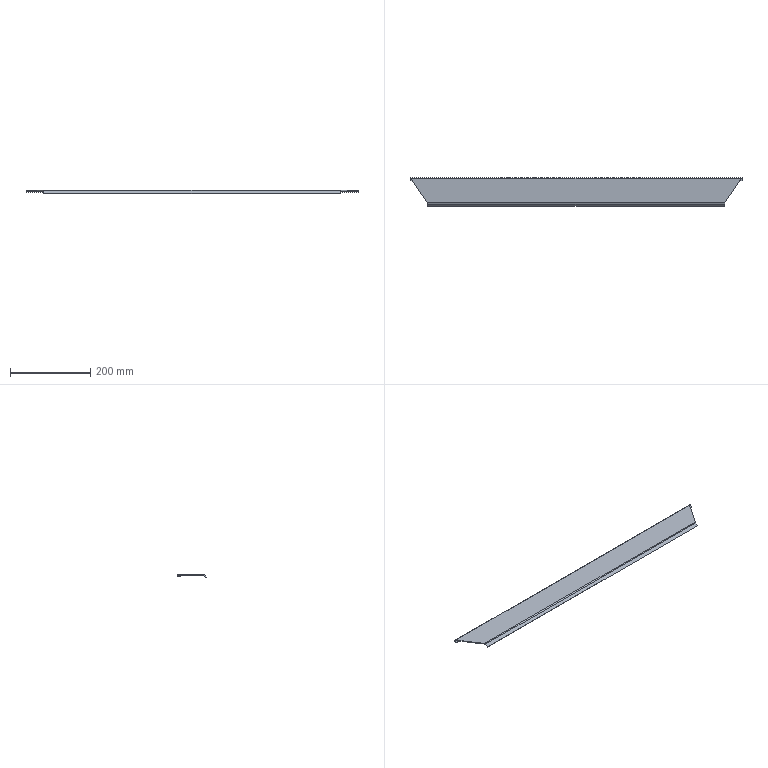Part | SolidWorks | features BaseBody 1 | 1 solid | 22 faces | box 828 x 72.071 x 8.485 mm | volume 128085 mm3 | plane 16 | cylinder 4 | spline 2 | commonest cylinder face diameters 1 x1 4 x1 5 x1 8 x1
STEP:
#1=CARTESIAN_POINT('',(371.122,-30.843,0.));
#2=VERTEX_POINT('',#1);
#3=CARTESIAN_POINT('',(412.308,30.,0.));
#4=VERTEX_POINT('',#3);
#5=CARTESIAN_POINT('',(371.122,-30.843,0.));
#6=DIRECTION('',(0.5606,0.8281,0.));
#7=VECTOR('',#6,1000.);
#8=LINE('',#5,#7);
#9=EDGE_CURVE('',#2,#4,#8,.T.);
#10=ORIENTED_EDGE('',*,*,#9,.F.);
#11=CARTESIAN_POINT('',(-371.122,-30.843,0.));
#12=VERTEX_POINT('',#11);
#13=CARTESIAN_POINT('',(0.,-30.843,0.));
#14=DIRECTION('',(1.,0.,0.));
#15=VECTOR('',#14,1000.);
#16=LINE('',#13,#15);
#17=EDGE_CURVE('',#12,#2,#16,.T.);
#18=ORIENTED_EDGE('',*,*,#17,.F.);
#19=CARTESIAN_POINT('',(-412.308,30.,0.));
#20=VERTEX_POINT('',#19);
#21=CARTESIAN_POINT('',(-412.308,30.,0.));
#22=DIRECTION('',(0.5606,-0.8281,0.));
#23=VECTOR('',#22,1000.);
#24=LINE('',#21,#23);
#25=EDGE_CURVE('',#20,#12,#24,.T.);
#26=ORIENTED_EDGE('',*,*,#25,.F.);
#27=CARTESIAN_POINT('',(0.,30.,0.));
#28=DIRECTION('',(-1.,0.,0.));
#29=VECTOR('',#28,1000.);
#30=LINE('',#27,#29);
#31=EDGE_CURVE('',#4,#20,#30,.T.);
#32=ORIENTED_EDGE('',*,*,#31,.F.);
#33=EDGE_LOOP('',(#10,#18,#26,#32));
#34=FACE_OUTER_BOUND('',#33,.T.);
#35=CARTESIAN_POINT('',(0.,1.658,0.));
#36=DIRECTION('',(0.,0.,1.));
#37=DIRECTION('',(1.,0.,0.));
#38=AXIS2_PLACEMENT_3D('',#35,#36,#37);
#39=PLANE('',#38);
#40=ADVANCED_FACE('',(#34),#39,.F.);
#41=CARTESIAN_POINT('',(414.,30.,0.));
#42=VERTEX_POINT('',#41);
#43=CARTESIAN_POINT('',(-414.,30.,0.));
#44=DIRECTION('',(1.,0.,0.));
#45=VECTOR('',#44,1000.);
#46=LINE('',#43,#45);
#47=EDGE_CURVE('',#4,#42,#46,.T.);
#48=ORIENTED_EDGE('',*,*,#47,.F.);
#49=ORIENTED_EDGE('',*,*,#31,.T.);
#50=CARTESIAN_POINT('',(-414.,30.,0.));
#51=VERTEX_POINT('',#50);
#52=CARTESIAN_POINT('',(-414.,30.,0.));
#53=DIRECTION('',(1.,0.,0.));
#54=VECTOR('',#53,1000.);
#55=LINE('',#52,#54);
#56=EDGE_CURVE('',#51,#20,#55,.T.);
#57=ORIENTED_EDGE('',*,*,#56,.F.);
#58=CARTESIAN_POINT('',(-414.,30.,-1.));
#59=VERTEX_POINT('',#58);
#60=CARTESIAN_POINT('',(-414.,30.,-0.5));
#61=DIRECTION('',(-1.,0.,0.));
#62=DIRECTION('',(0.,0.,-1.));
#63=AXIS2_PLACEMENT_3D('',#60,#61,#62);
#64=CIRCLE('',#63,0.5);
#65=EDGE_CURVE('',#51,#59,#64,.T.);
#66=ORIENTED_EDGE('',*,*,#65,.T.);
#67=CARTESIAN_POINT('',(414.,30.,-1.));
#68=VERTEX_POINT('',#67);
#69=CARTESIAN_POINT('',(-414.,30.,-1.));
#70=DIRECTION('',(-1.,0.,0.));
#71=VECTOR('',#70,1000.);
#72=LINE('',#69,#71);
#73=EDGE_CURVE('',#68,#59,#72,.T.);
#74=ORIENTED_EDGE('',*,*,#73,.F.);
#75=CARTESIAN_POINT('',(414.,30.,-0.5));
#76=DIRECTION('',(-1.,0.,0.));
#77=DIRECTION('',(0.,0.,-1.));
#78=AXIS2_PLACEMENT_3D('',#75,#76,#77);
#79=CIRCLE('',#78,0.5);
#80=EDGE_CURVE('',#42,#68,#79,.T.);
#81=ORIENTED_EDGE('',*,*,#80,.F.);
#82=EDGE_LOOP('',(#48,#49,#57,#66,#74,#81));
#83=FACE_OUTER_BOUND('',#82,.T.);
#84=CARTESIAN_POINT('',(-414.,30.,-0.5));
#85=DIRECTION('',(1.,0.,0.));
#86=DIRECTION('',(0.,0.,-1.));
#87=AXIS2_PLACEMENT_3D('',#84,#85,#86);
#88=CYLINDRICAL_SURFACE('',#87,0.5);
#89=ADVANCED_FACE('',(#83),#88,.F.);
#90=CARTESIAN_POINT('',(371.122,-30.843,2.));
#91=VERTEX_POINT('',#90);
#92=CARTESIAN_POINT('',(371.122,-30.843,0.));
#93=DIRECTION('',(0.,0.,-1.));
#94=VECTOR('',#93,1000.);
#95=LINE('',#92,#94);
#96=EDGE_CURVE('',#91,#2,#95,.T.);
#97=ORIENTED_EDGE('',*,*,#96,.T.);
#98=ORIENTED_EDGE('',*,*,#9,.T.);
#99=CARTESIAN_POINT('',(412.308,30.,2.));
#100=VERTEX_POINT('',#99);
#101=CARTESIAN_POINT('',(412.308,30.,0.));
#102=DIRECTION('',(0.,0.,1.));
#103=VECTOR('',#102,1000.);
#104=LINE('',#101,#103);
#105=EDGE_CURVE('',#4,#100,#104,.T.);
#106=ORIENTED_EDGE('',*,*,#105,.T.);
#107=CARTESIAN_POINT('',(414.,32.5,2.));
#108=DIRECTION('',(-0.5606,-0.8281,0.));
#109=VECTOR('',#108,1000.);
#110=LINE('',#107,#109);
#111=EDGE_CURVE('',#100,#91,#110,.T.);
#112=ORIENTED_EDGE('',*,*,#111,.T.);
#113=EDGE_LOOP('',(#97,#98,#106,#112));
#114=FACE_OUTER_BOUND('',#113,.T.);
#115=CARTESIAN_POINT('',(414.,32.5,0.));
#116=DIRECTION('',(0.8281,-0.5606,0.));
#117=DIRECTION('',(0.5606,0.8281,0.));
#118=AXIS2_PLACEMENT_3D('',#115,#116,#117);
#119=PLANE('',#118);
#120=ADVANCED_FACE('',(#114),#119,.T.);
#121=CARTESIAN_POINT('',(-370.,-32.257,-0.5858));
#122=VERTEX_POINT('',#121);
#123=CARTESIAN_POINT('',(-371.122,-30.843,0.));
#124=CARTESIAN_POINT('',(-370.934,-31.106,0.));
#125=CARTESIAN_POINT('',(-370.747,-31.368,-0.05216));
#126=CARTESIAN_POINT('',(-370.372,-31.853,-0.2539));
#127=CARTESIAN_POINT('',(-370.188,-32.071,-0.3997));
#128=CARTESIAN_POINT('',(-370.,-32.257,-0.5858));
#129=B_SPLINE_CURVE_WITH_KNOTS('',3,(#123,#124,#125,#126,#127,#128),.UNSPECIFIED.,.F.,.F.,(4,2,4),(0.,0.0009665,0.001933),.UNSPECIFIED.);
#130=EDGE_CURVE('',#12,#122,#129,.T.);
#131=ORIENTED_EDGE('',*,*,#130,.F.);
#132=ORIENTED_EDGE('',*,*,#17,.T.);
#133=CARTESIAN_POINT('',(370.,-32.257,-0.5858));
#134=VERTEX_POINT('',#133);
#135=CARTESIAN_POINT('',(370.,-32.257,-0.5858));
#136=CARTESIAN_POINT('',(370.188,-32.071,-0.3997));
#137=CARTESIAN_POINT('',(370.375,-31.85,-0.2518));
#138=CARTESIAN_POINT('',(370.75,-31.364,-0.05109));
#139=CARTESIAN_POINT('',(370.934,-31.106,0.));
#140=CARTESIAN_POINT('',(371.122,-30.843,0.));
#141=B_SPLINE_CURVE_WITH_KNOTS('',3,(#135,#136,#137,#138,#139,#140),.UNSPECIFIED.,.F.,.F.,(4,2,4),(0.,0.0009665,0.001933),.UNSPECIFIED.);
#142=EDGE_CURVE('',#134,#2,#141,.T.);
#143=ORIENTED_EDGE('',*,*,#142,.F.);
#144=CARTESIAN_POINT('',(0.,-32.257,-0.5858));
#145=DIRECTION('',(1.,0.,0.));
#146=VECTOR('',#145,1000.);
#147=LINE('',#144,#146);
#148=EDGE_CURVE('',#122,#134,#147,.T.);
#149=ORIENTED_EDGE('',*,*,#148,.F.);
#150=EDGE_LOOP('',(#131,#132,#143,#149));
#151=FACE_OUTER_BOUND('',#150,.T.);
#152=CARTESIAN_POINT('',(0.,-30.843,-2.));
#153=DIRECTION('',(1.,0.,0.));
#154=DIRECTION('',(0.,1.,0.));
#155=AXIS2_PLACEMENT_3D('',#152,#153,#154);
#156=CYLINDRICAL_SURFACE('',#155,2.);
#157=ADVANCED_FACE('',(#151),#156,.F.);
#158=CARTESIAN_POINT('',(-371.122,-30.843,2.));
#159=VERTEX_POINT('',#158);
#160=CARTESIAN_POINT('',(-371.122,-30.843,0.));
#161=DIRECTION('',(0.,0.,1.));
#162=VECTOR('',#161,1000.);
#163=LINE('',#160,#162);
#164=EDGE_CURVE('',#12,#159,#163,.T.);
#165=ORIENTED_EDGE('',*,*,#164,.T.);
#166=CARTESIAN_POINT('',(-412.308,30.,2.));
#167=VERTEX_POINT('',#166);
#168=CARTESIAN_POINT('',(-370.,-32.5,2.));
#169=DIRECTION('',(-0.5606,0.8281,0.));
#170=VECTOR('',#169,1000.);
#171=LINE('',#168,#170);
#172=EDGE_CURVE('',#159,#167,#171,.T.);
#173=ORIENTED_EDGE('',*,*,#172,.T.);
#174=CARTESIAN_POINT('',(-412.308,30.,0.));
#175=DIRECTION('',(0.,0.,-1.));
#176=VECTOR('',#175,1000.);
#177=LINE('',#174,#176);
#178=EDGE_CURVE('',#167,#20,#177,.T.);
#179=ORIENTED_EDGE('',*,*,#178,.T.);
#180=ORIENTED_EDGE('',*,*,#25,.T.);
#181=EDGE_LOOP('',(#165,#173,#179,#180));
#182=FACE_OUTER_BOUND('',#181,.T.);
#183=CARTESIAN_POINT('',(-370.,-32.5,0.));
#184=DIRECTION('',(-0.8281,-0.5606,0.));
#185=DIRECTION('',(0.5606,-0.8281,0.));
#186=AXIS2_PLACEMENT_3D('',#183,#184,#185);
#187=PLANE('',#186);
#188=ADVANCED_FACE('',(#182),#187,.T.);
#189=CARTESIAN_POINT('',(-414.,24.5,-1.));
#190=VERTEX_POINT('',#189);
#191=CARTESIAN_POINT('',(-414.,24.5,-1.));
#192=DIRECTION('',(0.,-1.,0.));
#193=VECTOR('',#192,1000.);
#194=LINE('',#191,#193);
#195=EDGE_CURVE('',#59,#190,#194,.T.);
#196=ORIENTED_EDGE('',*,*,#195,.T.);
#197=CARTESIAN_POINT('',(414.,24.5,-1.));
#198=VERTEX_POINT('',#197);
#199=CARTESIAN_POINT('',(-414.,24.5,-1.));
#200=DIRECTION('',(1.,0.,0.));
#201=VECTOR('',#200,1000.);
#202=LINE('',#199,#201);
#203=EDGE_CURVE('',#190,#198,#202,.T.);
#204=ORIENTED_EDGE('',*,*,#203,.T.);
#205=CARTESIAN_POINT('',(414.,24.5,-1.));
#206=DIRECTION('',(0.,1.,0.));
#207=VECTOR('',#206,1000.);
#208=LINE('',#205,#207);
#209=EDGE_CURVE('',#198,#68,#208,.T.);
#210=ORIENTED_EDGE('',*,*,#209,.T.);
#211=ORIENTED_EDGE('',*,*,#73,.T.);
#212=EDGE_LOOP('',(#196,#204,#210,#211));
#213=FACE_OUTER_BOUND('',#212,.T.);
#214=CARTESIAN_POINT('',(-414.,24.5,-1.));
#215=DIRECTION('',(0.,0.,1.));
#216=DIRECTION('',(0.,-1.,0.));
#217=AXIS2_PLACEMENT_3D('',#214,#215,#216);
#218=PLANE('',#217);
#219=ADVANCED_FACE('',(#213),#218,.T.);
#220=CARTESIAN_POINT('',(370.,-33.672,0.8284));
#221=VERTEX_POINT('',#220);
#222=CARTESIAN_POINT('',(371.122,-30.843,2.));
#223=CARTESIAN_POINT('',(371.027,-31.107,2.));
#224=CARTESIAN_POINT('',(370.934,-31.367,1.974));
#225=CARTESIAN_POINT('',(370.748,-31.878,1.873));
#226=CARTESIAN_POINT('',(370.655,-32.131,1.796));
#227=CARTESIAN_POINT('',(370.467,-32.616,1.595));
#228=CARTESIAN_POINT('',(370.375,-32.846,1.472));
#229=CARTESIAN_POINT('',(370.188,-33.28,1.183));
#230=CARTESIAN_POINT('',(370.094,-33.485,1.015));
#231=CARTESIAN_POINT('',(370.,-33.672,0.8284));
#232=B_SPLINE_CURVE_WITH_KNOTS('',3,(#222,#223,#224,#225,#226,#227,#228,#229,#230,#231),.UNSPECIFIED.,.F.,.F.,(4,2,2,2,4),(0.,0.0008293,0.001659,0.002488,0.003317),.UNSPECIFIED.);
#233=EDGE_CURVE('',#91,#221,#232,.T.);
#234=ORIENTED_EDGE('',*,*,#233,.T.);
#235=CARTESIAN_POINT('',(370.,-32.964,0.1213));
#236=DIRECTION('',(0.,0.7071,-0.7071));
#237=VECTOR('',#236,1000.);
#238=LINE('',#235,#237);
#239=EDGE_CURVE('',#221,#134,#238,.T.);
#240=ORIENTED_EDGE('',*,*,#239,.T.);
#241=ORIENTED_EDGE('',*,*,#142,.T.);
#242=ORIENTED_EDGE('',*,*,#96,.F.);
#243=EDGE_LOOP('',(#234,#240,#241,#242));
#244=FACE_OUTER_BOUND('',#243,.T.);
#245=CARTESIAN_POINT('',(370.,-33.686,0.8426));
#246=CARTESIAN_POINT('',(370.374,-32.942,1.587));
#247=CARTESIAN_POINT('',(370.748,-31.896,2.02));
#248=CARTESIAN_POINT('',(371.122,-30.843,2.02));
#249=CARTESIAN_POINT('',(370.,-33.681,0.8379));
#250=CARTESIAN_POINT('',(370.374,-32.938,1.581));
#251=CARTESIAN_POINT('',(370.748,-31.894,2.013));
#252=CARTESIAN_POINT('',(371.122,-30.843,2.013));
#253=CARTESIAN_POINT('',(370.,-33.676,0.8331));
#254=CARTESIAN_POINT('',(370.374,-32.935,1.575));
#255=CARTESIAN_POINT('',(370.748,-31.892,2.007));
#256=CARTESIAN_POINT('',(371.122,-30.843,2.007));
#257=CARTESIAN_POINT('',(370.,-33.672,0.8284));
#258=CARTESIAN_POINT('',(370.374,-32.931,1.569));
#259=CARTESIAN_POINT('',(370.748,-31.89,2.));
#260=CARTESIAN_POINT('',(371.122,-30.843,2.));
#261=CARTESIAN_POINT('',(370.,-33.2,0.357));
#262=CARTESIAN_POINT('',(370.374,-32.583,0.9741));
#263=CARTESIAN_POINT('',(370.748,-31.716,1.333));
#264=CARTESIAN_POINT('',(371.122,-30.843,1.333));
#265=CARTESIAN_POINT('',(370.,-32.729,-0.1144));
#266=CARTESIAN_POINT('',(370.374,-32.235,0.3793));
#267=CARTESIAN_POINT('',(370.748,-31.541,0.6667));
#268=CARTESIAN_POINT('',(371.122,-30.843,0.6667));
#269=CARTESIAN_POINT('',(370.,-32.257,-0.5858));
#270=CARTESIAN_POINT('',(370.374,-31.887,-0.2155));
#271=CARTESIAN_POINT('',(370.748,-31.367,0.));
#272=CARTESIAN_POINT('',(371.122,-30.843,0.));
#273=B_SPLINE_SURFACE_WITH_KNOTS('',3,3,((#245,#246,#247,#248),(#249,#250,#251,#252),(#253,#254,#255,#256),(#257,#258,#259,#260),(#261,#262,#263,#264),(#265,#266,#267,#268),(#269,#270,#271,#272)),.UNSPECIFIED.,.F.,.F.,.F.,(4,3,4),(4,4),(-0.002,0.,0.2),(0.,0.2525),.UNSPECIFIED.);
#274=ADVANCED_FACE('',(#244),#273,.T.);
#275=CARTESIAN_POINT('',(0.,-30.843,2.));
#276=DIRECTION('',(1.,0.,0.));
#277=VECTOR('',#276,1000.);
#278=LINE('',#275,#277);
#279=EDGE_CURVE('',#159,#91,#278,.T.);
#280=ORIENTED_EDGE('',*,*,#279,.T.);
#281=ORIENTED_EDGE('',*,*,#111,.F.);
#282=CARTESIAN_POINT('',(0.,30.,2.));
#283=DIRECTION('',(-1.,0.,0.));
#284=VECTOR('',#283,1000.);
#285=LINE('',#282,#284);
#286=EDGE_CURVE('',#100,#167,#285,.T.);
#287=ORIENTED_EDGE('',*,*,#286,.T.);
#288=ORIENTED_EDGE('',*,*,#172,.F.);
#289=EDGE_LOOP('',(#280,#281,#287,#288));
#290=FACE_OUTER_BOUND('',#289,.T.);
#291=CARTESIAN_POINT('',(0.,1.658,2.));
#292=DIRECTION('',(0.,0.,1.));
#293=DIRECTION('',(1.,0.,0.));
#294=AXIS2_PLACEMENT_3D('',#291,#292,#293);
#295=PLANE('',#294);
#296=ADVANCED_FACE('',(#290),#295,.T.);
#297=CARTESIAN_POINT('',(414.,30.,2.));
#298=VERTEX_POINT('',#297);
#299=CARTESIAN_POINT('',(414.,30.,0.));
#300=DIRECTION('',(0.,0.,1.));
#301=VECTOR('',#300,1000.);
#302=LINE('',#299,#301);
#303=EDGE_CURVE('',#42,#298,#302,.T.);
#304=ORIENTED_EDGE('',*,*,#303,.T.);
#305=CARTESIAN_POINT('',(-414.,30.,2.));
#306=DIRECTION('',(-1.,0.,0.));
#307=VECTOR('',#306,1000.);
#308=LINE('',#305,#307);
#309=EDGE_CURVE('',#298,#100,#308,.T.);
#310=ORIENTED_EDGE('',*,*,#309,.T.);
#311=ORIENTED_EDGE('',*,*,#105,.F.);
#312=ORIENTED_EDGE('',*,*,#47,.T.);
#313=EDGE_LOOP('',(#304,#310,#311,#312));
#314=FACE_OUTER_BOUND('',#313,.T.);
#315=CARTESIAN_POINT('',(-414.,30.,0.));
#316=DIRECTION('',(0.,-1.,0.));
#317=DIRECTION('',(0.,0.,-1.));
#318=AXIS2_PLACEMENT_3D('',#315,#316,#317);
#319=PLANE('',#318);
#320=ADVANCED_FACE('',(#314),#319,.T.);
#321=CARTESIAN_POINT('',(370.,-38.157,-6.485));
#322=VERTEX_POINT('',#321);
#323=CARTESIAN_POINT('',(370.,-34.401,-2.729));
#324=DIRECTION('',(0.,0.7071,0.7071));
#325=VECTOR('',#324,1000.);
#326=LINE('',#323,#325);
#327=EDGE_CURVE('',#322,#134,#326,.T.);
#328=ORIENTED_EDGE('',*,*,#327,.F.);
#329=CARTESIAN_POINT('',(-370.,-38.157,-6.485));
#330=VERTEX_POINT('',#329);
#331=CARTESIAN_POINT('',(0.,-38.157,-6.485));
#332=DIRECTION('',(1.,0.,0.));
#333=VECTOR('',#332,1000.);
#334=LINE('',#331,#333);
#335=EDGE_CURVE('',#330,#322,#334,.T.);
#336=ORIENTED_EDGE('',*,*,#335,.F.);
#337=CARTESIAN_POINT('',(-370.,-34.401,-2.729));
#338=DIRECTION('',(0.,-0.7071,-0.7071));
#339=VECTOR('',#338,1000.);
#340=LINE('',#337,#339);
#341=EDGE_CURVE('',#122,#330,#340,.T.);
#342=ORIENTED_EDGE('',*,*,#341,.F.);
#343=ORIENTED_EDGE('',*,*,#148,.T.);
#344=EDGE_LOOP('',(#328,#336,#342,#343));
#345=FACE_OUTER_BOUND('',#344,.T.);
#346=CARTESIAN_POINT('',(0.,-34.401,-2.729));
#347=DIRECTION('',(0.,-0.7071,0.7071));
#348=DIRECTION('',(0.,-0.7071,-0.7071));
#349=AXIS2_PLACEMENT_3D('',#346,#347,#348);
#350=PLANE('',#349);
#351=ADVANCED_FACE('',(#345),#350,.F.);
#352=ORIENTED_EDGE('',*,*,#164,.F.);
#353=ORIENTED_EDGE('',*,*,#130,.T.);
#354=CARTESIAN_POINT('',(-370.,-33.672,0.8284));
#355=VERTEX_POINT('',#354);
#356=CARTESIAN_POINT('',(-370.,-32.964,0.1213));
#357=DIRECTION('',(0.,-0.7071,0.7071));
#358=VECTOR('',#357,1000.);
#359=LINE('',#356,#358);
#360=EDGE_CURVE('',#122,#355,#359,.T.);
#361=ORIENTED_EDGE('',*,*,#360,.T.);
#362=CARTESIAN_POINT('',(-370.,-33.672,0.8284));
#363=CARTESIAN_POINT('',(-370.094,-33.485,1.015));
#364=CARTESIAN_POINT('',(-370.187,-33.283,1.181));
#365=CARTESIAN_POINT('',(-370.373,-32.85,1.47));
#366=CARTESIAN_POINT('',(-370.467,-32.617,1.595));
#367=CARTESIAN_POINT('',(-370.654,-32.131,1.796));
#368=CARTESIAN_POINT('',(-370.747,-31.882,1.872));
#369=CARTESIAN_POINT('',(-370.933,-31.371,1.974));
#370=CARTESIAN_POINT('',(-371.027,-31.107,2.));
#371=CARTESIAN_POINT('',(-371.122,-30.843,2.));
#372=B_SPLINE_CURVE_WITH_KNOTS('',3,(#362,#363,#364,#365,#366,#367,#368,#369,#370,#371),.UNSPECIFIED.,.F.,.F.,(4,2,2,2,4),(0.,0.0008293,0.001659,0.002488,0.003317),.UNSPECIFIED.);
#373=EDGE_CURVE('',#355,#159,#372,.T.);
#374=ORIENTED_EDGE('',*,*,#373,.T.);
#375=EDGE_LOOP('',(#352,#353,#361,#374));
#376=FACE_OUTER_BOUND('',#375,.T.);
#377=CARTESIAN_POINT('',(-370.,-32.257,-0.5858));
#378=CARTESIAN_POINT('',(-370.374,-31.887,-0.2155));
#379=CARTESIAN_POINT('',(-370.748,-31.367,0.));
#380=CARTESIAN_POINT('',(-371.122,-30.843,0.));
#381=CARTESIAN_POINT('',(-370.,-32.729,-0.1144));
#382=CARTESIAN_POINT('',(-370.374,-32.235,0.3793));
#383=CARTESIAN_POINT('',(-370.748,-31.541,0.6667));
#384=CARTESIAN_POINT('',(-371.122,-30.843,0.6667));
#385=CARTESIAN_POINT('',(-370.,-33.2,0.357));
#386=CARTESIAN_POINT('',(-370.374,-32.583,0.9741));
#387=CARTESIAN_POINT('',(-370.748,-31.716,1.333));
#388=CARTESIAN_POINT('',(-371.122,-30.843,1.333));
#389=CARTESIAN_POINT('',(-370.,-33.672,0.8284));
#390=CARTESIAN_POINT('',(-370.374,-32.931,1.569));
#391=CARTESIAN_POINT('',(-370.748,-31.89,2.));
#392=CARTESIAN_POINT('',(-371.122,-30.843,2.));
#393=CARTESIAN_POINT('',(-370.,-33.676,0.8331));
#394=CARTESIAN_POINT('',(-370.374,-32.935,1.575));
#395=CARTESIAN_POINT('',(-370.748,-31.892,2.007));
#396=CARTESIAN_POINT('',(-371.122,-30.843,2.007));
#397=CARTESIAN_POINT('',(-370.,-33.681,0.8379));
#398=CARTESIAN_POINT('',(-370.374,-32.938,1.581));
#399=CARTESIAN_POINT('',(-370.748,-31.894,2.013));
#400=CARTESIAN_POINT('',(-371.122,-30.843,2.013));
#401=CARTESIAN_POINT('',(-370.,-33.686,0.8426));
#402=CARTESIAN_POINT('',(-370.374,-32.942,1.587));
#403=CARTESIAN_POINT('',(-370.748,-31.896,2.02));
#404=CARTESIAN_POINT('',(-371.122,-30.843,2.02));
#405=B_SPLINE_SURFACE_WITH_KNOTS('',3,3,((#377,#378,#379,#380),(#381,#382,#383,#384),(#385,#386,#387,#388),(#389,#390,#391,#392),(#393,#394,#395,#396),(#397,#398,#399,#400),(#401,#402,#403,#404)),.UNSPECIFIED.,.F.,.F.,.F.,(4,3,4),(4,4),(-0.2,0.,0.002),(-0.2525,0.),.UNSPECIFIED.);
#406=ADVANCED_FACE('',(#376),#405,.T.);
#407=CARTESIAN_POINT('',(-414.,30.,2.));
#408=VERTEX_POINT('',#407);
#409=CARTESIAN_POINT('',(-414.,30.,0.));
#410=DIRECTION('',(0.,0.,-1.));
#411=VECTOR('',#410,1000.);
#412=LINE('',#409,#411);
#413=EDGE_CURVE('',#408,#51,#412,.T.);
#414=ORIENTED_EDGE('',*,*,#413,.T.);
#415=ORIENTED_EDGE('',*,*,#56,.T.);
#416=ORIENTED_EDGE('',*,*,#178,.F.);
#417=CARTESIAN_POINT('',(-414.,30.,2.));
#418=DIRECTION('',(-1.,0.,0.));
#419=VECTOR('',#418,1000.);
#420=LINE('',#417,#419);
#421=EDGE_CURVE('',#167,#408,#420,.T.);
#422=ORIENTED_EDGE('',*,*,#421,.T.);
#423=EDGE_LOOP('',(#414,#415,#416,#422));
#424=FACE_OUTER_BOUND('',#423,.T.);
#425=CARTESIAN_POINT('',(-414.,30.,0.));
#426=DIRECTION('',(0.,-1.,0.));
#427=DIRECTION('',(0.,0.,-1.));
#428=AXIS2_PLACEMENT_3D('',#425,#426,#427);
#429=PLANE('',#428);
#430=ADVANCED_FACE('',(#424),#429,.T.);
#431=CARTESIAN_POINT('',(-414.,24.5,-3.));
#432=VERTEX_POINT('',#431);
#433=CARTESIAN_POINT('',(-414.,24.5,-3.));
#434=DIRECTION('',(0.,0.,-1.));
#435=VECTOR('',#434,1000.);
#436=LINE('',#433,#435);
#437=EDGE_CURVE('',#190,#432,#436,.T.);
#438=ORIENTED_EDGE('',*,*,#437,.T.);
#439=CARTESIAN_POINT('',(414.,24.5,-3.));
#440=VERTEX_POINT('',#439);
#441=CARTESIAN_POINT('',(-414.,24.5,-3.));
#442=DIRECTION('',(1.,0.,0.));
#443=VECTOR('',#442,1000.);
#444=LINE('',#441,#443);
#445=EDGE_CURVE('',#432,#440,#444,.T.);
#446=ORIENTED_EDGE('',*,*,#445,.T.);
#447=CARTESIAN_POINT('',(414.,24.5,-3.));
#448=DIRECTION('',(0.,0.,1.));
#449=VECTOR('',#448,1000.);
#450=LINE('',#447,#449);
#451=EDGE_CURVE('',#440,#198,#450,.T.);
#452=ORIENTED_EDGE('',*,*,#451,.T.);
#453=ORIENTED_EDGE('',*,*,#203,.F.);
#454=EDGE_LOOP('',(#438,#446,#452,#453));
#455=FACE_OUTER_BOUND('',#454,.T.);
#456=CARTESIAN_POINT('',(-414.,24.5,-3.));
#457=DIRECTION('',(0.,-1.,0.));
#458=DIRECTION('',(0.,0.,-1.));
#459=AXIS2_PLACEMENT_3D('',#456,#457,#458);
#460=PLANE('',#459);
#461=ADVANCED_FACE('',(#455),#460,.T.);
#462=CARTESIAN_POINT('',(-414.,30.,-3.));
#463=VERTEX_POINT('',#462);
#464=CARTESIAN_POINT('',(-414.,28.791,-3.));
#465=DIRECTION('',(0.,1.,0.));
#466=VECTOR('',#465,1000.);
#467=LINE('',#464,#466);
#468=EDGE_CURVE('',#432,#463,#467,.T.);
#469=ORIENTED_EDGE('',*,*,#468,.F.);
#470=ORIENTED_EDGE('',*,*,#437,.F.);
#471=ORIENTED_EDGE('',*,*,#195,.F.);
#472=ORIENTED_EDGE('',*,*,#65,.F.);
#473=ORIENTED_EDGE('',*,*,#413,.F.);
#474=CARTESIAN_POINT('',(-414.,30.,-0.5));
#475=DIRECTION('',(1.,0.,0.));
#476=DIRECTION('',(0.,0.,-1.));
#477=AXIS2_PLACEMENT_3D('',#474,#475,#476);
#478=CIRCLE('',#477,2.5);
#479=EDGE_CURVE('',#463,#408,#478,.T.);
#480=ORIENTED_EDGE('',*,*,#479,.F.);
#481=EDGE_LOOP('',(#469,#470,#471,#472,#473,#480));
#482=FACE_OUTER_BOUND('',#481,.T.);
#483=CARTESIAN_POINT('',(-414.,28.791,-1.176));
#484=DIRECTION('',(1.,0.,0.));
#485=DIRECTION('',(0.,1.,0.));
#486=AXIS2_PLACEMENT_3D('',#483,#484,#485);
#487=PLANE('',#486);
#488=ADVANCED_FACE('',(#482),#487,.F.);
#489=ORIENTED_EDGE('',*,*,#451,.F.);
#490=CARTESIAN_POINT('',(414.,30.,-3.));
#491=VERTEX_POINT('',#490);
#492=CARTESIAN_POINT('',(414.,28.791,-3.));
#493=DIRECTION('',(0.,1.,0.));
#494=VECTOR('',#493,1000.);
#495=LINE('',#492,#494);
#496=EDGE_CURVE('',#440,#491,#495,.T.);
#497=ORIENTED_EDGE('',*,*,#496,.T.);
#498=CARTESIAN_POINT('',(414.,30.,-0.5));
#499=DIRECTION('',(-1.,0.,0.));
#500=DIRECTION('',(0.,0.,-1.));
#501=AXIS2_PLACEMENT_3D('',#498,#499,#500);
#502=CIRCLE('',#501,2.5);
#503=EDGE_CURVE('',#298,#491,#502,.T.);
#504=ORIENTED_EDGE('',*,*,#503,.F.);
#505=ORIENTED_EDGE('',*,*,#303,.F.);
#506=ORIENTED_EDGE('',*,*,#80,.T.);
#507=ORIENTED_EDGE('',*,*,#209,.F.);
#508=EDGE_LOOP('',(#489,#497,#504,#505,#506,#507));
#509=FACE_OUTER_BOUND('',#508,.T.);
#510=CARTESIAN_POINT('',(414.,28.791,-1.176));
#511=DIRECTION('',(1.,0.,0.));
#512=DIRECTION('',(0.,0.,-1.));
#513=AXIS2_PLACEMENT_3D('',#510,#511,#512);
#514=PLANE('',#513);
#515=ADVANCED_FACE('',(#509),#514,.T.);
#516=CARTESIAN_POINT('',(370.,-39.571,-5.071));
#517=VERTEX_POINT('',#516);
#518=CARTESIAN_POINT('',(370.,-33.672,0.8284));
#519=DIRECTION('',(0.,-0.7071,-0.7071));
#520=VECTOR('',#519,1000.);
#521=LINE('',#518,#520);
#522=EDGE_CURVE('',#221,#517,#521,.T.);
#523=ORIENTED_EDGE('',*,*,#522,.T.);
#524=CARTESIAN_POINT('',(370.,-39.571,-5.071));
#525=DIRECTION('',(0.,0.7071,-0.7071));
#526=VECTOR('',#525,1000.);
#527=LINE('',#524,#526);
#528=EDGE_CURVE('',#517,#322,#527,.T.);
#529=ORIENTED_EDGE('',*,*,#528,.T.);
#530=ORIENTED_EDGE('',*,*,#327,.T.);
#531=ORIENTED_EDGE('',*,*,#239,.F.);
#532=EDGE_LOOP('',(#523,#529,#530,#531));
#533=FACE_OUTER_BOUND('',#532,.T.);
#534=CARTESIAN_POINT('',(370.,-39.571,-5.071));
#535=DIRECTION('',(1.,0.,0.));
#536=DIRECTION('',(0.,0.,-1.));
#537=AXIS2_PLACEMENT_3D('',#534,#535,#536);
#538=PLANE('',#537);
#539=ADVANCED_FACE('',(#533),#538,.T.);
#540=ORIENTED_EDGE('',*,*,#279,.F.);
#541=ORIENTED_EDGE('',*,*,#373,.F.);
#542=CARTESIAN_POINT('',(0.,-33.672,0.8284));
#543=DIRECTION('',(1.,0.,0.));
#544=VECTOR('',#543,1000.);
#545=LINE('',#542,#544);
#546=EDGE_CURVE('',#355,#221,#545,.T.);
#547=ORIENTED_EDGE('',*,*,#546,.T.);
#548=ORIENTED_EDGE('',*,*,#233,.F.);
#549=EDGE_LOOP('',(#540,#541,#547,#548));
#550=FACE_OUTER_BOUND('',#549,.T.);
#551=CARTESIAN_POINT('',(0.,-30.843,-2.));
#552=DIRECTION('',(1.,0.,0.));
#553=DIRECTION('',(0.,1.,0.));
#554=AXIS2_PLACEMENT_3D('',#551,#552,#553);
#555=CYLINDRICAL_SURFACE('',#554,4.);
#556=ADVANCED_FACE('',(#550),#555,.T.);
#557=ORIENTED_EDGE('',*,*,#286,.F.);
#558=ORIENTED_EDGE('',*,*,#309,.F.);
#559=ORIENTED_EDGE('',*,*,#503,.T.);
#560=CARTESIAN_POINT('',(-414.,30.,-3.));
#561=DIRECTION('',(-1.,0.,0.));
#562=VECTOR('',#561,1000.);
#563=LINE('',#560,#562);
#564=EDGE_CURVE('',#491,#463,#563,.T.);
#565=ORIENTED_EDGE('',*,*,#564,.T.);
#566=ORIENTED_EDGE('',*,*,#479,.T.);
#567=ORIENTED_EDGE('',*,*,#421,.F.);
#568=EDGE_LOOP('',(#557,#558,#559,#565,#566,#567));
#569=FACE_OUTER_BOUND('',#568,.T.);
#570=CARTESIAN_POINT('',(-414.,30.,-0.5));
#571=DIRECTION('',(1.,0.,0.));
#572=DIRECTION('',(0.,0.,-1.));
#573=AXIS2_PLACEMENT_3D('',#570,#571,#572);
#574=CYLINDRICAL_SURFACE('',#573,2.5);
#575=ADVANCED_FACE('',(#569),#574,.T.);
#576=CARTESIAN_POINT('',(-370.,-39.571,-5.071));
#577=VERTEX_POINT('',#576);
#578=CARTESIAN_POINT('',(-370.,-39.571,-5.071));
#579=DIRECTION('',(-1.,0.,0.));
#580=VECTOR('',#579,1000.);
#581=LINE('',#578,#580);
#582=EDGE_CURVE('',#517,#577,#581,.T.);
#583=ORIENTED_EDGE('',*,*,#582,.T.);
#584=CARTESIAN_POINT('',(-370.,-39.571,-5.071));
#585=DIRECTION('',(0.,0.7071,-0.7071));
#586=VECTOR('',#585,1000.);
#587=LINE('',#584,#586);
#588=EDGE_CURVE('',#577,#330,#587,.T.);
#589=ORIENTED_EDGE('',*,*,#588,.T.);
#590=ORIENTED_EDGE('',*,*,#335,.T.);
#591=ORIENTED_EDGE('',*,*,#528,.F.);
#592=EDGE_LOOP('',(#583,#589,#590,#591));
#593=FACE_OUTER_BOUND('',#592,.T.);
#594=CARTESIAN_POINT('',(-370.,-39.571,-5.071));
#595=DIRECTION('',(0.,-0.7071,-0.7071));
#596=DIRECTION('',(0.,0.7071,-0.7071));
#597=AXIS2_PLACEMENT_3D('',#594,#595,#596);
#598=PLANE('',#597);
#599=ADVANCED_FACE('',(#593),#598,.T.);
#600=CARTESIAN_POINT('',(-370.,-39.571,-5.071));
#601=DIRECTION('',(0.,0.7071,0.7071));
#602=VECTOR('',#601,1000.);
#603=LINE('',#600,#602);
#604=EDGE_CURVE('',#577,#355,#603,.T.);
#605=ORIENTED_EDGE('',*,*,#604,.T.);
#606=ORIENTED_EDGE('',*,*,#360,.F.);
#607=ORIENTED_EDGE('',*,*,#341,.T.);
#608=ORIENTED_EDGE('',*,*,#588,.F.);
#609=EDGE_LOOP('',(#605,#606,#607,#608));
#610=FACE_OUTER_BOUND('',#609,.T.);
#611=CARTESIAN_POINT('',(-370.,-33.672,0.8284));
#612=DIRECTION('',(-1.,0.,0.));
#613=DIRECTION('',(0.,0.,1.));
#614=AXIS2_PLACEMENT_3D('',#611,#612,#613);
#615=PLANE('',#614);
#616=ADVANCED_FACE('',(#610),#615,.T.);
#617=ORIENTED_EDGE('',*,*,#468,.T.);
#618=ORIENTED_EDGE('',*,*,#564,.F.);
#619=ORIENTED_EDGE('',*,*,#496,.F.);
#620=ORIENTED_EDGE('',*,*,#445,.F.);
#621=EDGE_LOOP('',(#617,#618,#619,#620));
#622=FACE_OUTER_BOUND('',#621,.T.);
#623=CARTESIAN_POINT('',(-414.,30.,-3.));
#624=DIRECTION('',(0.,0.,-1.));
#625=DIRECTION('',(0.,1.,0.));
#626=AXIS2_PLACEMENT_3D('',#623,#624,#625);
#627=PLANE('',#626);
#628=ADVANCED_FACE('',(#622),#627,.T.);
#629=ORIENTED_EDGE('',*,*,#582,.F.);
#630=ORIENTED_EDGE('',*,*,#522,.F.);
#631=ORIENTED_EDGE('',*,*,#546,.F.);
#632=ORIENTED_EDGE('',*,*,#604,.F.);
#633=EDGE_LOOP('',(#629,#630,#631,#632));
#634=FACE_OUTER_BOUND('',#633,.T.);
#635=CARTESIAN_POINT('',(0.,-35.815,-1.315));
#636=DIRECTION('',(0.,-0.7071,0.7071));
#637=DIRECTION('',(0.,-0.7071,-0.7071));
#638=AXIS2_PLACEMENT_3D('',#635,#636,#637);
#639=PLANE('',#638);
#640=ADVANCED_FACE('',(#634),#639,.T.);
#641=CLOSED_SHELL('',(#40,#89,#120,#157,#188,#219,#274,#296,#320,#351,#406,#430,#461,#488,#515,#539,#556,#575,#599,#616,#628,#640));
#642=MANIFOLD_SOLID_BREP('',#641);
#643=CARTESIAN_POINT('',(0.,0.,0.));
#644=DIRECTION('',(0.,0.,1.));
#645=DIRECTION('',(1.,0.,0.));
#646=AXIS2_PLACEMENT_3D('',#643,#644,#645);
#647=(LENGTH_UNIT()NAMED_UNIT(*)SI_UNIT(.MILLI.,.METRE.));
#648=UNCERTAINTY_MEASURE_WITH_UNIT(LENGTH_MEASURE(0.00001),#647,'','');
#649=(NAMED_UNIT(*)PLANE_ANGLE_UNIT()SI_UNIT($,.RADIAN.));
#650=(NAMED_UNIT(*)SI_UNIT($,.STERADIAN.)SOLID_ANGLE_UNIT());
#651=(GEOMETRIC_REPRESENTATION_CONTEXT(3)GLOBAL_UNCERTAINTY_ASSIGNED_CONTEXT((#648))GLOBAL_UNIT_ASSIGNED_CONTEXT((#647,#649,#650))REPRESENTATION_CONTEXT('',''));
#652=ADVANCED_BREP_SHAPE_REPRESENTATION('',(#642,#646),#651);